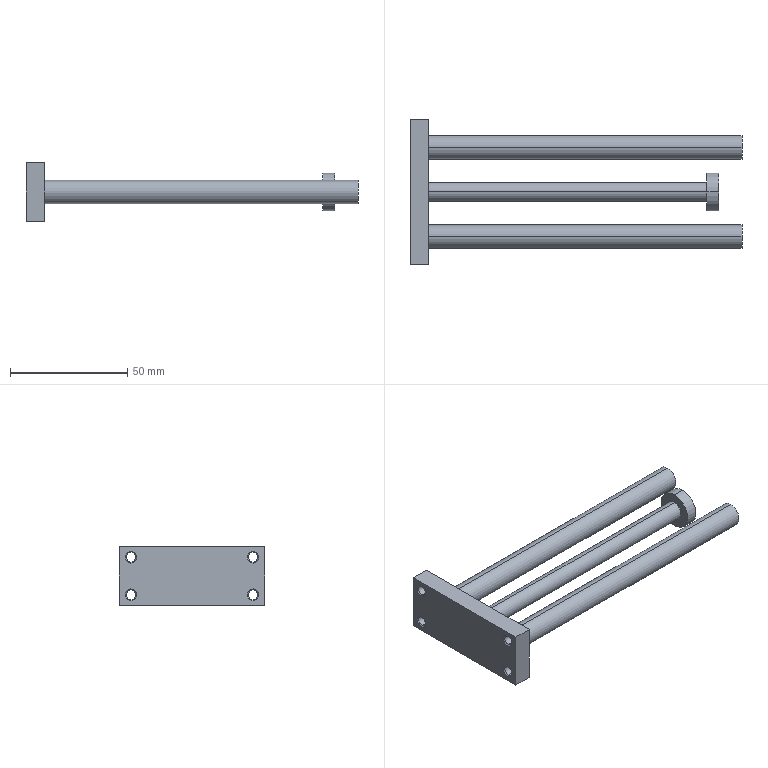Part | SolidWorks | features RefAxis 3, LPattern 2, Revolution 2, 3DProfileFeature 1, Extrusion 1, RevCut 1 | 1 solid | 42 faces | box 141.5 x 62 x 25 mm | volume 39892 mm3 | cylinder 16 | cone 16 | plane 10 | commonest cylinder face diameters 4.134 x8 10 x4 8 x2 16 x2
STEP:
#1=CARTESIAN_POINT('',(123.5,0.,8.));
#2=VERTEX_POINT('',#1);
#3=CARTESIAN_POINT('',(123.5,0.,-8.));
#4=VERTEX_POINT('',#3);
#5=CARTESIAN_POINT('',(123.5,0.,0.));
#6=DIRECTION('',(-1.,0.,0.));
#7=DIRECTION('',(0.,0.,1.));
#8=AXIS2_PLACEMENT_3D('',#5,#6,#7);
#9=CIRCLE('',#8,8.);
#10=EDGE_CURVE('',#2,#4,#9,.T.);
#11=ORIENTED_EDGE('',*,*,#10,.T.);
#12=CARTESIAN_POINT('',(118.5,0.,-8.));
#13=VERTEX_POINT('',#12);
#14=CARTESIAN_POINT('',(123.5,0.,-8.));
#15=DIRECTION('',(-1.,0.,0.));
#16=VECTOR('',#15,1000.);
#17=LINE('',#14,#16);
#18=EDGE_CURVE('',#4,#13,#17,.T.);
#19=ORIENTED_EDGE('',*,*,#18,.T.);
#20=CARTESIAN_POINT('',(118.5,0.,8.));
#21=VERTEX_POINT('',#20);
#22=CARTESIAN_POINT('',(118.5,0.,0.));
#23=DIRECTION('',(-1.,0.,0.));
#24=DIRECTION('',(0.,0.,1.));
#25=AXIS2_PLACEMENT_3D('',#22,#23,#24);
#26=CIRCLE('',#25,8.);
#27=EDGE_CURVE('',#21,#13,#26,.T.);
#28=ORIENTED_EDGE('',*,*,#27,.F.);
#29=CARTESIAN_POINT('',(123.5,0.,8.));
#30=DIRECTION('',(-1.,0.,0.));
#31=VECTOR('',#30,1000.);
#32=LINE('',#29,#31);
#33=EDGE_CURVE('',#2,#21,#32,.T.);
#34=ORIENTED_EDGE('',*,*,#33,.F.);
#35=EDGE_LOOP('',(#11,#19,#28,#34));
#36=FACE_OUTER_BOUND('',#35,.T.);
#37=CARTESIAN_POINT('',(123.5,0.,0.));
#38=DIRECTION('',(-1.,0.,0.));
#39=DIRECTION('',(0.,0.,1.));
#40=AXIS2_PLACEMENT_3D('',#37,#38,#39);
#41=CYLINDRICAL_SURFACE('',#40,8.);
#42=ADVANCED_FACE('',(#36),#41,.T.);
#43=CARTESIAN_POINT('',(118.5,0.,4.));
#44=VERTEX_POINT('',#43);
#45=CARTESIAN_POINT('',(118.5,0.,-4.));
#46=VERTEX_POINT('',#45);
#47=CARTESIAN_POINT('',(118.5,0.,0.));
#48=DIRECTION('',(-1.,0.,0.));
#49=DIRECTION('',(0.,0.,1.));
#50=AXIS2_PLACEMENT_3D('',#47,#48,#49);
#51=CIRCLE('',#50,4.);
#52=EDGE_CURVE('',#44,#46,#51,.T.);
#53=ORIENTED_EDGE('',*,*,#52,.T.);
#54=CARTESIAN_POINT('',(0.,0.,-4.));
#55=VERTEX_POINT('',#54);
#56=CARTESIAN_POINT('',(123.5,0.,-4.));
#57=DIRECTION('',(-1.,0.,0.));
#58=VECTOR('',#57,1000.);
#59=LINE('',#56,#58);
#60=EDGE_CURVE('',#46,#55,#59,.T.);
#61=ORIENTED_EDGE('',*,*,#60,.T.);
#62=CARTESIAN_POINT('',(0.,0.,4.));
#63=VERTEX_POINT('',#62);
#64=CARTESIAN_POINT('',(0.,0.,0.));
#65=DIRECTION('',(-1.,0.,0.));
#66=DIRECTION('',(0.,0.,1.));
#67=AXIS2_PLACEMENT_3D('',#64,#65,#66);
#68=CIRCLE('',#67,4.);
#69=EDGE_CURVE('',#63,#55,#68,.T.);
#70=ORIENTED_EDGE('',*,*,#69,.F.);
#71=CARTESIAN_POINT('',(123.5,0.,4.));
#72=DIRECTION('',(-1.,0.,0.));
#73=VECTOR('',#72,1000.);
#74=LINE('',#71,#73);
#75=EDGE_CURVE('',#44,#63,#74,.T.);
#76=ORIENTED_EDGE('',*,*,#75,.F.);
#77=EDGE_LOOP('',(#53,#61,#70,#76));
#78=FACE_OUTER_BOUND('',#77,.T.);
#79=CARTESIAN_POINT('',(123.5,0.,0.));
#80=DIRECTION('',(-1.,0.,0.));
#81=DIRECTION('',(0.,0.,1.));
#82=AXIS2_PLACEMENT_3D('',#79,#80,#81);
#83=CYLINDRICAL_SURFACE('',#82,4.);
#84=ADVANCED_FACE('',(#78),#83,.T.);
#85=CARTESIAN_POINT('',(-0.433,-26.,-10.067));
#86=VERTEX_POINT('',#85);
#87=CARTESIAN_POINT('',(-0.433,-26.,-5.933));
#88=VERTEX_POINT('',#87);
#89=CARTESIAN_POINT('',(-0.433,-26.,-8.));
#90=DIRECTION('',(-1.,0.,0.));
#91=DIRECTION('',(0.,0.,1.));
#92=AXIS2_PLACEMENT_3D('',#89,#90,#91);
#93=CIRCLE('',#92,2.067);
#94=EDGE_CURVE('',#86,#88,#93,.T.);
#95=ORIENTED_EDGE('',*,*,#94,.T.);
#96=CARTESIAN_POINT('',(0.,-26.,-5.5));
#97=VERTEX_POINT('',#96);
#98=CARTESIAN_POINT('',(0.,-26.,-5.5));
#99=DIRECTION('',(0.7071,0.,0.7071));
#100=VECTOR('',#99,1000.);
#101=LINE('',#98,#100);
#102=EDGE_CURVE('',#88,#97,#101,.T.);
#103=ORIENTED_EDGE('',*,*,#102,.T.);
#104=CARTESIAN_POINT('',(0.,-26.,-10.5));
#105=VERTEX_POINT('',#104);
#106=CARTESIAN_POINT('',(0.,-26.,-8.));
#107=DIRECTION('',(-1.,0.,0.));
#108=DIRECTION('',(0.,0.,1.));
#109=AXIS2_PLACEMENT_3D('',#106,#107,#108);
#110=CIRCLE('',#109,2.5);
#111=EDGE_CURVE('',#105,#97,#110,.T.);
#112=ORIENTED_EDGE('',*,*,#111,.F.);
#113=CARTESIAN_POINT('',(0.,-26.,-10.5));
#114=DIRECTION('',(0.7071,0.,-0.7071));
#115=VECTOR('',#114,1000.);
#116=LINE('',#113,#115);
#117=EDGE_CURVE('',#86,#105,#116,.T.);
#118=ORIENTED_EDGE('',*,*,#117,.F.);
#119=EDGE_LOOP('',(#95,#103,#112,#118));
#120=FACE_OUTER_BOUND('',#119,.T.);
#121=CARTESIAN_POINT('',(0.,-26.,-8.));
#122=DIRECTION('',(1.,0.,0.));
#123=DIRECTION('',(0.,0.,-1.));
#124=AXIS2_PLACEMENT_3D('',#121,#122,#123);
#125=CONICAL_SURFACE('',#124,2.5,0.7854);
#126=ADVANCED_FACE('',(#120),#125,.F.);
#127=ORIENTED_EDGE('',*,*,#94,.F.);
#128=CARTESIAN_POINT('',(-7.567,-26.,-10.067));
#129=VERTEX_POINT('',#128);
#130=CARTESIAN_POINT('',(0.,-26.,-10.067));
#131=DIRECTION('',(-1.,0.,0.));
#132=VECTOR('',#131,1000.);
#133=LINE('',#130,#132);
#134=EDGE_CURVE('',#86,#129,#133,.T.);
#135=ORIENTED_EDGE('',*,*,#134,.T.);
#136=CARTESIAN_POINT('',(-7.567,-26.,-5.933));
#137=VERTEX_POINT('',#136);
#138=CARTESIAN_POINT('',(-7.567,-26.,-8.));
#139=DIRECTION('',(-1.,0.,0.));
#140=DIRECTION('',(0.,0.,1.));
#141=AXIS2_PLACEMENT_3D('',#138,#139,#140);
#142=CIRCLE('',#141,2.067);
#143=EDGE_CURVE('',#129,#137,#142,.T.);
#144=ORIENTED_EDGE('',*,*,#143,.T.);
#145=CARTESIAN_POINT('',(0.,-26.,-5.933));
#146=DIRECTION('',(-1.,0.,0.));
#147=VECTOR('',#146,1000.);
#148=LINE('',#145,#147);
#149=EDGE_CURVE('',#88,#137,#148,.T.);
#150=ORIENTED_EDGE('',*,*,#149,.F.);
#151=EDGE_LOOP('',(#127,#135,#144,#150));
#152=FACE_OUTER_BOUND('',#151,.T.);
#153=CARTESIAN_POINT('',(0.,-26.,-8.));
#154=DIRECTION('',(-1.,0.,0.));
#155=DIRECTION('',(0.,0.,1.));
#156=AXIS2_PLACEMENT_3D('',#153,#154,#155);
#157=CYLINDRICAL_SURFACE('',#156,2.067);
#158=ADVANCED_FACE('',(#152),#157,.F.);
#159=ORIENTED_EDGE('',*,*,#143,.F.);
#160=CARTESIAN_POINT('',(-8.,-26.,-10.5));
#161=VERTEX_POINT('',#160);
#162=CARTESIAN_POINT('',(-7.567,-26.,-10.067));
#163=DIRECTION('',(-0.7071,0.,-0.7071));
#164=VECTOR('',#163,1000.);
#165=LINE('',#162,#164);
#166=EDGE_CURVE('',#129,#161,#165,.T.);
#167=ORIENTED_EDGE('',*,*,#166,.T.);
#168=CARTESIAN_POINT('',(-8.,-26.,-5.5));
#169=VERTEX_POINT('',#168);
#170=CARTESIAN_POINT('',(-8.,-26.,-8.));
#171=DIRECTION('',(-1.,0.,0.));
#172=DIRECTION('',(0.,0.,1.));
#173=AXIS2_PLACEMENT_3D('',#170,#171,#172);
#174=CIRCLE('',#173,2.5);
#175=EDGE_CURVE('',#161,#169,#174,.T.);
#176=ORIENTED_EDGE('',*,*,#175,.T.);
#177=CARTESIAN_POINT('',(-7.567,-26.,-5.933));
#178=DIRECTION('',(-0.7071,0.,0.7071));
#179=VECTOR('',#178,1000.);
#180=LINE('',#177,#179);
#181=EDGE_CURVE('',#137,#169,#180,.T.);
#182=ORIENTED_EDGE('',*,*,#181,.F.);
#183=EDGE_LOOP('',(#159,#167,#176,#182));
#184=FACE_OUTER_BOUND('',#183,.T.);
#185=CARTESIAN_POINT('',(-7.567,-26.,-8.));
#186=DIRECTION('',(-1.,0.,0.));
#187=DIRECTION('',(0.,0.,1.));
#188=AXIS2_PLACEMENT_3D('',#185,#186,#187);
#189=CONICAL_SURFACE('',#188,2.067,0.7854);
#190=ADVANCED_FACE('',(#184),#189,.F.);
#191=CARTESIAN_POINT('',(-0.433,26.,-10.067));
#192=VERTEX_POINT('',#191);
#193=CARTESIAN_POINT('',(-0.433,26.,-5.933));
#194=VERTEX_POINT('',#193);
#195=CARTESIAN_POINT('',(-0.433,26.,-8.));
#196=DIRECTION('',(-1.,0.,0.));
#197=DIRECTION('',(0.,0.,1.));
#198=AXIS2_PLACEMENT_3D('',#195,#196,#197);
#199=CIRCLE('',#198,2.067);
#200=EDGE_CURVE('',#192,#194,#199,.T.);
#201=ORIENTED_EDGE('',*,*,#200,.T.);
#202=CARTESIAN_POINT('',(0.,26.,-5.5));
#203=VERTEX_POINT('',#202);
#204=CARTESIAN_POINT('',(0.,26.,-5.5));
#205=DIRECTION('',(0.7071,0.,0.7071));
#206=VECTOR('',#205,1000.);
#207=LINE('',#204,#206);
#208=EDGE_CURVE('',#194,#203,#207,.T.);
#209=ORIENTED_EDGE('',*,*,#208,.T.);
#210=CARTESIAN_POINT('',(0.,26.,-10.5));
#211=VERTEX_POINT('',#210);
#212=CARTESIAN_POINT('',(0.,26.,-8.));
#213=DIRECTION('',(-1.,0.,0.));
#214=DIRECTION('',(0.,0.,1.));
#215=AXIS2_PLACEMENT_3D('',#212,#213,#214);
#216=CIRCLE('',#215,2.5);
#217=EDGE_CURVE('',#211,#203,#216,.T.);
#218=ORIENTED_EDGE('',*,*,#217,.F.);
#219=CARTESIAN_POINT('',(0.,26.,-10.5));
#220=DIRECTION('',(0.7071,0.,-0.7071));
#221=VECTOR('',#220,1000.);
#222=LINE('',#219,#221);
#223=EDGE_CURVE('',#192,#211,#222,.T.);
#224=ORIENTED_EDGE('',*,*,#223,.F.);
#225=EDGE_LOOP('',(#201,#209,#218,#224));
#226=FACE_OUTER_BOUND('',#225,.T.);
#227=CARTESIAN_POINT('',(0.,26.,-8.));
#228=DIRECTION('',(1.,0.,0.));
#229=DIRECTION('',(0.,0.,-1.));
#230=AXIS2_PLACEMENT_3D('',#227,#228,#229);
#231=CONICAL_SURFACE('',#230,2.5,0.7854);
#232=ADVANCED_FACE('',(#226),#231,.F.);
#233=ORIENTED_EDGE('',*,*,#200,.F.);
#234=CARTESIAN_POINT('',(-7.567,26.,-10.067));
#235=VERTEX_POINT('',#234);
#236=CARTESIAN_POINT('',(0.,26.,-10.067));
#237=DIRECTION('',(-1.,0.,0.));
#238=VECTOR('',#237,1000.);
#239=LINE('',#236,#238);
#240=EDGE_CURVE('',#192,#235,#239,.T.);
#241=ORIENTED_EDGE('',*,*,#240,.T.);
#242=CARTESIAN_POINT('',(-7.567,26.,-5.933));
#243=VERTEX_POINT('',#242);
#244=CARTESIAN_POINT('',(-7.567,26.,-8.));
#245=DIRECTION('',(-1.,0.,0.));
#246=DIRECTION('',(0.,0.,1.));
#247=AXIS2_PLACEMENT_3D('',#244,#245,#246);
#248=CIRCLE('',#247,2.067);
#249=EDGE_CURVE('',#235,#243,#248,.T.);
#250=ORIENTED_EDGE('',*,*,#249,.T.);
#251=CARTESIAN_POINT('',(0.,26.,-5.933));
#252=DIRECTION('',(-1.,0.,0.));
#253=VECTOR('',#252,1000.);
#254=LINE('',#251,#253);
#255=EDGE_CURVE('',#194,#243,#254,.T.);
#256=ORIENTED_EDGE('',*,*,#255,.F.);
#257=EDGE_LOOP('',(#233,#241,#250,#256));
#258=FACE_OUTER_BOUND('',#257,.T.);
#259=CARTESIAN_POINT('',(0.,26.,-8.));
#260=DIRECTION('',(-1.,0.,0.));
#261=DIRECTION('',(0.,0.,1.));
#262=AXIS2_PLACEMENT_3D('',#259,#260,#261);
#263=CYLINDRICAL_SURFACE('',#262,2.067);
#264=ADVANCED_FACE('',(#258),#263,.F.);
#265=ORIENTED_EDGE('',*,*,#249,.F.);
#266=CARTESIAN_POINT('',(-8.,26.,-10.5));
#267=VERTEX_POINT('',#266);
#268=CARTESIAN_POINT('',(-7.567,26.,-10.067));
#269=DIRECTION('',(-0.7071,0.,-0.7071));
#270=VECTOR('',#269,1000.);
#271=LINE('',#268,#270);
#272=EDGE_CURVE('',#235,#267,#271,.T.);
#273=ORIENTED_EDGE('',*,*,#272,.T.);
#274=CARTESIAN_POINT('',(-8.,26.,-5.5));
#275=VERTEX_POINT('',#274);
#276=CARTESIAN_POINT('',(-8.,26.,-8.));
#277=DIRECTION('',(-1.,0.,0.));
#278=DIRECTION('',(0.,0.,1.));
#279=AXIS2_PLACEMENT_3D('',#276,#277,#278);
#280=CIRCLE('',#279,2.5);
#281=EDGE_CURVE('',#267,#275,#280,.T.);
#282=ORIENTED_EDGE('',*,*,#281,.T.);
#283=CARTESIAN_POINT('',(-7.567,26.,-5.933));
#284=DIRECTION('',(-0.7071,0.,0.7071));
#285=VECTOR('',#284,1000.);
#286=LINE('',#283,#285);
#287=EDGE_CURVE('',#243,#275,#286,.T.);
#288=ORIENTED_EDGE('',*,*,#287,.F.);
#289=EDGE_LOOP('',(#265,#273,#282,#288));
#290=FACE_OUTER_BOUND('',#289,.T.);
#291=CARTESIAN_POINT('',(-7.567,26.,-8.));
#292=DIRECTION('',(-1.,0.,0.));
#293=DIRECTION('',(0.,0.,1.));
#294=AXIS2_PLACEMENT_3D('',#291,#292,#293);
#295=CONICAL_SURFACE('',#294,2.067,0.7854);
#296=ADVANCED_FACE('',(#290),#295,.F.);
#297=CARTESIAN_POINT('',(-0.433,-26.,5.933));
#298=VERTEX_POINT('',#297);
#299=CARTESIAN_POINT('',(-0.433,-26.,10.067));
#300=VERTEX_POINT('',#299);
#301=CARTESIAN_POINT('',(-0.433,-26.,8.));
#302=DIRECTION('',(-1.,0.,0.));
#303=DIRECTION('',(0.,0.,1.));
#304=AXIS2_PLACEMENT_3D('',#301,#302,#303);
#305=CIRCLE('',#304,2.067);
#306=EDGE_CURVE('',#298,#300,#305,.T.);
#307=ORIENTED_EDGE('',*,*,#306,.T.);
#308=CARTESIAN_POINT('',(0.,-26.,10.5));
#309=VERTEX_POINT('',#308);
#310=CARTESIAN_POINT('',(0.,-26.,10.5));
#311=DIRECTION('',(0.7071,0.,0.7071));
#312=VECTOR('',#311,1000.);
#313=LINE('',#310,#312);
#314=EDGE_CURVE('',#300,#309,#313,.T.);
#315=ORIENTED_EDGE('',*,*,#314,.T.);
#316=CARTESIAN_POINT('',(0.,-26.,5.5));
#317=VERTEX_POINT('',#316);
#318=CARTESIAN_POINT('',(0.,-26.,8.));
#319=DIRECTION('',(-1.,0.,0.));
#320=DIRECTION('',(0.,0.,1.));
#321=AXIS2_PLACEMENT_3D('',#318,#319,#320);
#322=CIRCLE('',#321,2.5);
#323=EDGE_CURVE('',#317,#309,#322,.T.);
#324=ORIENTED_EDGE('',*,*,#323,.F.);
#325=CARTESIAN_POINT('',(0.,-26.,5.5));
#326=DIRECTION('',(0.7071,0.,-0.7071));
#327=VECTOR('',#326,1000.);
#328=LINE('',#325,#327);
#329=EDGE_CURVE('',#298,#317,#328,.T.);
#330=ORIENTED_EDGE('',*,*,#329,.F.);
#331=EDGE_LOOP('',(#307,#315,#324,#330));
#332=FACE_OUTER_BOUND('',#331,.T.);
#333=CARTESIAN_POINT('',(0.,-26.,8.));
#334=DIRECTION('',(1.,0.,0.));
#335=DIRECTION('',(0.,0.,-1.));
#336=AXIS2_PLACEMENT_3D('',#333,#334,#335);
#337=CONICAL_SURFACE('',#336,2.5,0.7854);
#338=ADVANCED_FACE('',(#332),#337,.F.);
#339=ORIENTED_EDGE('',*,*,#306,.F.);
#340=CARTESIAN_POINT('',(-7.567,-26.,5.933));
#341=VERTEX_POINT('',#340);
#342=CARTESIAN_POINT('',(0.,-26.,5.933));
#343=DIRECTION('',(-1.,0.,0.));
#344=VECTOR('',#343,1000.);
#345=LINE('',#342,#344);
#346=EDGE_CURVE('',#298,#341,#345,.T.);
#347=ORIENTED_EDGE('',*,*,#346,.T.);
#348=CARTESIAN_POINT('',(-7.567,-26.,10.067));
#349=VERTEX_POINT('',#348);
#350=CARTESIAN_POINT('',(-7.567,-26.,8.));
#351=DIRECTION('',(-1.,0.,0.));
#352=DIRECTION('',(0.,0.,1.));
#353=AXIS2_PLACEMENT_3D('',#350,#351,#352);
#354=CIRCLE('',#353,2.067);
#355=EDGE_CURVE('',#341,#349,#354,.T.);
#356=ORIENTED_EDGE('',*,*,#355,.T.);
#357=CARTESIAN_POINT('',(0.,-26.,10.067));
#358=DIRECTION('',(-1.,0.,0.));
#359=VECTOR('',#358,1000.);
#360=LINE('',#357,#359);
#361=EDGE_CURVE('',#300,#349,#360,.T.);
#362=ORIENTED_EDGE('',*,*,#361,.F.);
#363=EDGE_LOOP('',(#339,#347,#356,#362));
#364=FACE_OUTER_BOUND('',#363,.T.);
#365=CARTESIAN_POINT('',(0.,-26.,8.));
#366=DIRECTION('',(-1.,0.,0.));
#367=DIRECTION('',(0.,0.,1.));
#368=AXIS2_PLACEMENT_3D('',#365,#366,#367);
#369=CYLINDRICAL_SURFACE('',#368,2.067);
#370=ADVANCED_FACE('',(#364),#369,.F.);
#371=ORIENTED_EDGE('',*,*,#355,.F.);
#372=CARTESIAN_POINT('',(-8.,-26.,5.5));
#373=VERTEX_POINT('',#372);
#374=CARTESIAN_POINT('',(-7.567,-26.,5.933));
#375=DIRECTION('',(-0.7071,0.,-0.7071));
#376=VECTOR('',#375,1000.);
#377=LINE('',#374,#376);
#378=EDGE_CURVE('',#341,#373,#377,.T.);
#379=ORIENTED_EDGE('',*,*,#378,.T.);
#380=CARTESIAN_POINT('',(-8.,-26.,10.5));
#381=VERTEX_POINT('',#380);
#382=CARTESIAN_POINT('',(-8.,-26.,8.));
#383=DIRECTION('',(-1.,0.,0.));
#384=DIRECTION('',(0.,0.,1.));
#385=AXIS2_PLACEMENT_3D('',#382,#383,#384);
#386=CIRCLE('',#385,2.5);
#387=EDGE_CURVE('',#373,#381,#386,.T.);
#388=ORIENTED_EDGE('',*,*,#387,.T.);
#389=CARTESIAN_POINT('',(-7.567,-26.,10.067));
#390=DIRECTION('',(-0.7071,0.,0.7071));
#391=VECTOR('',#390,1000.);
#392=LINE('',#389,#391);
#393=EDGE_CURVE('',#349,#381,#392,.T.);
#394=ORIENTED_EDGE('',*,*,#393,.F.);
#395=EDGE_LOOP('',(#371,#379,#388,#394));
#396=FACE_OUTER_BOUND('',#395,.T.);
#397=CARTESIAN_POINT('',(-7.567,-26.,8.));
#398=DIRECTION('',(-1.,0.,0.));
#399=DIRECTION('',(0.,0.,1.));
#400=AXIS2_PLACEMENT_3D('',#397,#398,#399);
#401=CONICAL_SURFACE('',#400,2.067,0.7854);
#402=ADVANCED_FACE('',(#396),#401,.F.);
#403=CARTESIAN_POINT('',(-0.433,26.,5.933));
#404=VERTEX_POINT('',#403);
#405=CARTESIAN_POINT('',(-0.433,26.,10.067));
#406=VERTEX_POINT('',#405);
#407=CARTESIAN_POINT('',(-0.433,26.,8.));
#408=DIRECTION('',(-1.,0.,0.));
#409=DIRECTION('',(0.,0.,1.));
#410=AXIS2_PLACEMENT_3D('',#407,#408,#409);
#411=CIRCLE('',#410,2.067);
#412=EDGE_CURVE('',#404,#406,#411,.T.);
#413=ORIENTED_EDGE('',*,*,#412,.T.);
#414=CARTESIAN_POINT('',(0.,26.,10.5));
#415=VERTEX_POINT('',#414);
#416=CARTESIAN_POINT('',(0.,26.,10.5));
#417=DIRECTION('',(0.7071,0.,0.7071));
#418=VECTOR('',#417,1000.);
#419=LINE('',#416,#418);
#420=EDGE_CURVE('',#406,#415,#419,.T.);
#421=ORIENTED_EDGE('',*,*,#420,.T.);
#422=CARTESIAN_POINT('',(0.,26.,5.5));
#423=VERTEX_POINT('',#422);
#424=CARTESIAN_POINT('',(0.,26.,8.));
#425=DIRECTION('',(-1.,0.,0.));
#426=DIRECTION('',(0.,0.,1.));
#427=AXIS2_PLACEMENT_3D('',#424,#425,#426);
#428=CIRCLE('',#427,2.5);
#429=EDGE_CURVE('',#423,#415,#428,.T.);
#430=ORIENTED_EDGE('',*,*,#429,.F.);
#431=CARTESIAN_POINT('',(0.,26.,5.5));
#432=DIRECTION('',(0.7071,0.,-0.7071));
#433=VECTOR('',#432,1000.);
#434=LINE('',#431,#433);
#435=EDGE_CURVE('',#404,#423,#434,.T.);
#436=ORIENTED_EDGE('',*,*,#435,.F.);
#437=EDGE_LOOP('',(#413,#421,#430,#436));
#438=FACE_OUTER_BOUND('',#437,.T.);
#439=CARTESIAN_POINT('',(0.,26.,8.));
#440=DIRECTION('',(1.,0.,0.));
#441=DIRECTION('',(0.,0.,-1.));
#442=AXIS2_PLACEMENT_3D('',#439,#440,#441);
#443=CONICAL_SURFACE('',#442,2.5,0.7854);
#444=ADVANCED_FACE('',(#438),#443,.F.);
#445=ORIENTED_EDGE('',*,*,#412,.F.);
#446=CARTESIAN_POINT('',(-7.567,26.,5.933));
#447=VERTEX_POINT('',#446);
#448=CARTESIAN_POINT('',(0.,26.,5.933));
#449=DIRECTION('',(-1.,0.,0.));
#450=VECTOR('',#449,1000.);
#451=LINE('',#448,#450);
#452=EDGE_CURVE('',#404,#447,#451,.T.);
#453=ORIENTED_EDGE('',*,*,#452,.T.);
#454=CARTESIAN_POINT('',(-7.567,26.,10.067));
#455=VERTEX_POINT('',#454);
#456=CARTESIAN_POINT('',(-7.567,26.,8.));
#457=DIRECTION('',(-1.,0.,0.));
#458=DIRECTION('',(0.,0.,1.));
#459=AXIS2_PLACEMENT_3D('',#456,#457,#458);
#460=CIRCLE('',#459,2.067);
#461=EDGE_CURVE('',#447,#455,#460,.T.);
#462=ORIENTED_EDGE('',*,*,#461,.T.);
#463=CARTESIAN_POINT('',(0.,26.,10.067));
#464=DIRECTION('',(-1.,0.,0.));
#465=VECTOR('',#464,1000.);
#466=LINE('',#463,#465);
#467=EDGE_CURVE('',#406,#455,#466,.T.);
#468=ORIENTED_EDGE('',*,*,#467,.F.);
#469=EDGE_LOOP('',(#445,#453,#462,#468));
#470=FACE_OUTER_BOUND('',#469,.T.);
#471=CARTESIAN_POINT('',(0.,26.,8.));
#472=DIRECTION('',(-1.,0.,0.));
#473=DIRECTION('',(0.,0.,1.));
#474=AXIS2_PLACEMENT_3D('',#471,#472,#473);
#475=CYLINDRICAL_SURFACE('',#474,2.067);
#476=ADVANCED_FACE('',(#470),#475,.F.);
#477=ORIENTED_EDGE('',*,*,#461,.F.);
#478=CARTESIAN_POINT('',(-8.,26.,5.5));
#479=VERTEX_POINT('',#478);
#480=CARTESIAN_POINT('',(-7.567,26.,5.933));
#481=DIRECTION('',(-0.7071,0.,-0.7071));
#482=VECTOR('',#481,1000.);
#483=LINE('',#480,#482);
#484=EDGE_CURVE('',#447,#479,#483,.T.);
#485=ORIENTED_EDGE('',*,*,#484,.T.);
#486=CARTESIAN_POINT('',(-8.,26.,10.5));
#487=VERTEX_POINT('',#486);
#488=CARTESIAN_POINT('',(-8.,26.,8.));
#489=DIRECTION('',(-1.,0.,0.));
#490=DIRECTION('',(0.,0.,1.));
#491=AXIS2_PLACEMENT_3D('',#488,#489,#490);
#492=CIRCLE('',#491,2.5);
#493=EDGE_CURVE('',#479,#487,#492,.T.);
#494=ORIENTED_EDGE('',*,*,#493,.T.);
#495=CARTESIAN_POINT('',(-7.567,26.,10.067));
#496=DIRECTION('',(-0.7071,0.,0.7071));
#497=VECTOR('',#496,1000.);
#498=LINE('',#495,#497);
#499=EDGE_CURVE('',#455,#487,#498,.T.);
#500=ORIENTED_EDGE('',*,*,#499,.F.);
#501=EDGE_LOOP('',(#477,#485,#494,#500));
#502=FACE_OUTER_BOUND('',#501,.T.);
#503=CARTESIAN_POINT('',(-7.567,26.,8.));
#504=DIRECTION('',(-1.,0.,0.));
#505=DIRECTION('',(0.,0.,1.));
#506=AXIS2_PLACEMENT_3D('',#503,#504,#505);
#507=CONICAL_SURFACE('',#506,2.067,0.7854);
#508=ADVANCED_FACE('',(#502),#507,.F.);
#509=CARTESIAN_POINT('',(133.5,-19.,5.));
#510=VERTEX_POINT('',#509);
#511=CARTESIAN_POINT('',(133.5,-19.,-5.));
#512=VERTEX_POINT('',#511);
#513=CARTESIAN_POINT('',(133.5,-19.,0.));
#514=DIRECTION('',(-1.,0.,0.));
#515=DIRECTION('',(0.,0.,1.));
#516=AXIS2_PLACEMENT_3D('',#513,#514,#515);
#517=CIRCLE('',#516,5.);
#518=EDGE_CURVE('',#510,#512,#517,.T.);
#519=ORIENTED_EDGE('',*,*,#518,.T.);
#520=CARTESIAN_POINT('',(0.,-19.,-5.));
#521=VERTEX_POINT('',#520);
#522=CARTESIAN_POINT('',(133.5,-19.,-5.));
#523=DIRECTION('',(-1.,0.,0.));
#524=VECTOR('',#523,1000.);
#525=LINE('',#522,#524);
#526=EDGE_CURVE('',#512,#521,#525,.T.);
#527=ORIENTED_EDGE('',*,*,#526,.T.);
#528=CARTESIAN_POINT('',(0.,-19.,5.));
#529=VERTEX_POINT('',#528);
#530=CARTESIAN_POINT('',(0.,-19.,0.));
#531=DIRECTION('',(-1.,0.,0.));
#532=DIRECTION('',(0.,0.,1.));
#533=AXIS2_PLACEMENT_3D('',#530,#531,#532);
#534=CIRCLE('',#533,5.);
#535=EDGE_CURVE('',#529,#521,#534,.T.);
#536=ORIENTED_EDGE('',*,*,#535,.F.);
#537=CARTESIAN_POINT('',(133.5,-19.,5.));
#538=DIRECTION('',(-1.,0.,0.));
#539=VECTOR('',#538,1000.);
#540=LINE('',#537,#539);
#541=EDGE_CURVE('',#510,#529,#540,.T.);
#542=ORIENTED_EDGE('',*,*,#541,.F.);
#543=EDGE_LOOP('',(#519,#527,#536,#542));
#544=FACE_OUTER_BOUND('',#543,.T.);
#545=CARTESIAN_POINT('',(133.5,-19.,0.));
#546=DIRECTION('',(-1.,0.,0.));
#547=DIRECTION('',(0.,0.,1.));
#548=AXIS2_PLACEMENT_3D('',#545,#546,#547);
#549=CYLINDRICAL_SURFACE('',#548,5.);
#550=ADVANCED_FACE('',(#544),#549,.T.);
#551=CARTESIAN_POINT('',(133.5,19.,5.));
#552=VERTEX_POINT('',#551);
#553=CARTESIAN_POINT('',(133.5,19.,-5.));
#554=VERTEX_POINT('',#553);
#555=CARTESIAN_POINT('',(133.5,19.,0.));
#556=DIRECTION('',(-1.,0.,0.));
#557=DIRECTION('',(0.,0.,1.));
#558=AXIS2_PLACEMENT_3D('',#555,#556,#557);
#559=CIRCLE('',#558,5.);
#560=EDGE_CURVE('',#552,#554,#559,.T.);
#561=ORIENTED_EDGE('',*,*,#560,.T.);
#562=CARTESIAN_POINT('',(0.,19.,-5.));
#563=VERTEX_POINT('',#562);
#564=CARTESIAN_POINT('',(133.5,19.,-5.));
#565=DIRECTION('',(-1.,0.,0.));
#566=VECTOR('',#565,1000.);
#567=LINE('',#564,#566);
#568=EDGE_CURVE('',#554,#563,#567,.T.);
#569=ORIENTED_EDGE('',*,*,#568,.T.);
#570=CARTESIAN_POINT('',(0.,19.,5.));
#571=VERTEX_POINT('',#570);
#572=CARTESIAN_POINT('',(0.,19.,0.));
#573=DIRECTION('',(-1.,0.,0.));
#574=DIRECTION('',(0.,0.,1.));
#575=AXIS2_PLACEMENT_3D('',#572,#573,#574);
#576=CIRCLE('',#575,5.);
#577=EDGE_CURVE('',#571,#563,#576,.T.);
#578=ORIENTED_EDGE('',*,*,#577,.F.);
#579=CARTESIAN_POINT('',(133.5,19.,5.));
#580=DIRECTION('',(-1.,0.,0.));
#581=VECTOR('',#580,1000.);
#582=LINE('',#579,#581);
#583=EDGE_CURVE('',#552,#571,#582,.T.);
#584=ORIENTED_EDGE('',*,*,#583,.F.);
#585=EDGE_LOOP('',(#561,#569,#578,#584));
#586=FACE_OUTER_BOUND('',#585,.T.);
#587=CARTESIAN_POINT('',(133.5,19.,0.));
#588=DIRECTION('',(-1.,0.,0.));
#589=DIRECTION('',(0.,0.,1.));
#590=AXIS2_PLACEMENT_3D('',#587,#588,#589);
#591=CYLINDRICAL_SURFACE('',#590,5.);
#592=ADVANCED_FACE('',(#586),#591,.T.);
#593=ORIENTED_EDGE('',*,*,#111,.T.);
#594=CARTESIAN_POINT('',(0.,-26.,-8.));
#595=DIRECTION('',(-1.,0.,0.));
#596=DIRECTION('',(0.,0.,1.));
#597=AXIS2_PLACEMENT_3D('',#594,#595,#596);
#598=CIRCLE('',#597,2.5);
#599=EDGE_CURVE('',#97,#105,#598,.T.);
#600=ORIENTED_EDGE('',*,*,#599,.T.);
#601=EDGE_LOOP('',(#593,#600));
#602=FACE_BOUND('',#601,.T.);
#603=ORIENTED_EDGE('',*,*,#323,.T.);
#604=CARTESIAN_POINT('',(0.,-26.,8.));
#605=DIRECTION('',(-1.,0.,0.));
#606=DIRECTION('',(0.,0.,1.));
#607=AXIS2_PLACEMENT_3D('',#604,#605,#606);
#608=CIRCLE('',#607,2.5);
#609=EDGE_CURVE('',#309,#317,#608,.T.);
#610=ORIENTED_EDGE('',*,*,#609,.T.);
#611=EDGE_LOOP('',(#603,#610));
#612=FACE_BOUND('',#611,.T.);
#613=ORIENTED_EDGE('',*,*,#535,.T.);
#614=CARTESIAN_POINT('',(0.,-19.,0.));
#615=DIRECTION('',(-1.,0.,0.));
#616=DIRECTION('',(0.,0.,1.));
#617=AXIS2_PLACEMENT_3D('',#614,#615,#616);
#618=CIRCLE('',#617,5.);
#619=EDGE_CURVE('',#521,#529,#618,.T.);
#620=ORIENTED_EDGE('',*,*,#619,.T.);
#621=EDGE_LOOP('',(#613,#620));
#622=FACE_BOUND('',#621,.T.);
#623=CARTESIAN_POINT('',(0.,31.,12.5));
#624=VERTEX_POINT('',#623);
#625=CARTESIAN_POINT('',(0.,-31.,12.5));
#626=VERTEX_POINT('',#625);
#627=CARTESIAN_POINT('',(0.,31.,12.5));
#628=DIRECTION('',(0.,-1.,0.));
#629=VECTOR('',#628,1000.);
#630=LINE('',#627,#629);
#631=EDGE_CURVE('',#624,#626,#630,.T.);
#632=ORIENTED_EDGE('',*,*,#631,.T.);
#633=CARTESIAN_POINT('',(0.,-31.,-12.5));
#634=VERTEX_POINT('',#633);
#635=CARTESIAN_POINT('',(0.,-31.,12.5));
#636=DIRECTION('',(0.,0.,-1.));
#637=VECTOR('',#636,1000.);
#638=LINE('',#635,#637);
#639=EDGE_CURVE('',#626,#634,#638,.T.);
#640=ORIENTED_EDGE('',*,*,#639,.T.);
#641=CARTESIAN_POINT('',(0.,31.,-12.5));
#642=VERTEX_POINT('',#641);
#643=CARTESIAN_POINT('',(0.,-31.,-12.5));
#644=DIRECTION('',(0.,1.,0.));
#645=VECTOR('',#644,1000.);
#646=LINE('',#643,#645);
#647=EDGE_CURVE('',#634,#642,#646,.T.);
#648=ORIENTED_EDGE('',*,*,#647,.T.);
#649=CARTESIAN_POINT('',(0.,31.,-12.5));
#650=DIRECTION('',(0.,0.,1.));
#651=VECTOR('',#650,1000.);
#652=LINE('',#649,#651);
#653=EDGE_CURVE('',#642,#624,#652,.T.);
#654=ORIENTED_EDGE('',*,*,#653,.T.);
#655=EDGE_LOOP('',(#632,#640,#648,#654));
#656=FACE_OUTER_BOUND('',#655,.T.);
#657=ORIENTED_EDGE('',*,*,#577,.T.);
#658=CARTESIAN_POINT('',(0.,19.,0.));
#659=DIRECTION('',(-1.,0.,0.));
#660=DIRECTION('',(0.,0.,1.));
#661=AXIS2_PLACEMENT_3D('',#658,#659,#660);
#662=CIRCLE('',#661,5.);
#663=EDGE_CURVE('',#563,#571,#662,.T.);
#664=ORIENTED_EDGE('',*,*,#663,.T.);
#665=EDGE_LOOP('',(#657,#664));
#666=FACE_BOUND('',#665,.T.);
#667=ORIENTED_EDGE('',*,*,#429,.T.);
#668=CARTESIAN_POINT('',(0.,26.,8.));
#669=DIRECTION('',(-1.,0.,0.));
#670=DIRECTION('',(0.,0.,1.));
#671=AXIS2_PLACEMENT_3D('',#668,#669,#670);
#672=CIRCLE('',#671,2.5);
#673=EDGE_CURVE('',#415,#423,#672,.T.);
#674=ORIENTED_EDGE('',*,*,#673,.T.);
#675=EDGE_LOOP('',(#667,#674));
#676=FACE_BOUND('',#675,.T.);
#677=ORIENTED_EDGE('',*,*,#217,.T.);
#678=CARTESIAN_POINT('',(0.,26.,-8.));
#679=DIRECTION('',(-1.,0.,0.));
#680=DIRECTION('',(0.,0.,1.));
#681=AXIS2_PLACEMENT_3D('',#678,#679,#680);
#682=CIRCLE('',#681,2.5);
#683=EDGE_CURVE('',#203,#211,#682,.T.);
#684=ORIENTED_EDGE('',*,*,#683,.T.);
#685=EDGE_LOOP('',(#677,#684));
#686=FACE_BOUND('',#685,.T.);
#687=ORIENTED_EDGE('',*,*,#69,.T.);
#688=CARTESIAN_POINT('',(0.,0.,0.));
#689=DIRECTION('',(-1.,0.,0.));
#690=DIRECTION('',(0.,0.,1.));
#691=AXIS2_PLACEMENT_3D('',#688,#689,#690);
#692=CIRCLE('',#691,4.);
#693=EDGE_CURVE('',#55,#63,#692,.T.);
#694=ORIENTED_EDGE('',*,*,#693,.T.);
#695=EDGE_LOOP('',(#687,#694));
#696=FACE_BOUND('',#695,.T.);
#697=CARTESIAN_POINT('',(0.,0.,0.));
#698=DIRECTION('',(1.,0.,0.));
#699=DIRECTION('',(0.,0.,-1.));
#700=AXIS2_PLACEMENT_3D('',#697,#698,#699);
#701=PLANE('',#700);
#702=ADVANCED_FACE('',(#602,#612,#622,#656,#666,#676,#686,#696),#701,.T.);
#703=CARTESIAN_POINT('',(-8.,26.,-8.));
#704=DIRECTION('',(-1.,0.,0.));
#705=DIRECTION('',(0.,0.,1.));
#706=AXIS2_PLACEMENT_3D('',#703,#704,#705);
#707=CIRCLE('',#706,2.5);
#708=EDGE_CURVE('',#275,#267,#707,.T.);
#709=ORIENTED_EDGE('',*,*,#708,.F.);
#710=ORIENTED_EDGE('',*,*,#281,.F.);
#711=EDGE_LOOP('',(#709,#710));
#712=FACE_BOUND('',#711,.T.);
#713=CARTESIAN_POINT('',(-8.,26.,8.));
#714=DIRECTION('',(-1.,0.,0.));
#715=DIRECTION('',(0.,0.,1.));
#716=AXIS2_PLACEMENT_3D('',#713,#714,#715);
#717=CIRCLE('',#716,2.5);
#718=EDGE_CURVE('',#487,#479,#717,.T.);
#719=ORIENTED_EDGE('',*,*,#718,.F.);
#720=ORIENTED_EDGE('',*,*,#493,.F.);
#721=EDGE_LOOP('',(#719,#720));
#722=FACE_BOUND('',#721,.T.);
#723=CARTESIAN_POINT('',(-8.,31.,12.5));
#724=VERTEX_POINT('',#723);
#725=CARTESIAN_POINT('',(-8.,-31.,12.5));
#726=VERTEX_POINT('',#725);
#727=CARTESIAN_POINT('',(-8.,31.,12.5));
#728=DIRECTION('',(0.,-1.,0.));
#729=VECTOR('',#728,1000.);
#730=LINE('',#727,#729);
#731=EDGE_CURVE('',#724,#726,#730,.T.);
#732=ORIENTED_EDGE('',*,*,#731,.F.);
#733=CARTESIAN_POINT('',(-8.,31.,-12.5));
#734=VERTEX_POINT('',#733);
#735=CARTESIAN_POINT('',(-8.,31.,-12.5));
#736=DIRECTION('',(0.,0.,1.));
#737=VECTOR('',#736,1000.);
#738=LINE('',#735,#737);
#739=EDGE_CURVE('',#734,#724,#738,.T.);
#740=ORIENTED_EDGE('',*,*,#739,.F.);
#741=CARTESIAN_POINT('',(-8.,-31.,-12.5));
#742=VERTEX_POINT('',#741);
#743=CARTESIAN_POINT('',(-8.,-31.,-12.5));
#744=DIRECTION('',(0.,1.,0.));
#745=VECTOR('',#744,1000.);
#746=LINE('',#743,#745);
#747=EDGE_CURVE('',#742,#734,#746,.T.);
#748=ORIENTED_EDGE('',*,*,#747,.F.);
#749=CARTESIAN_POINT('',(-8.,-31.,12.5));
#750=DIRECTION('',(0.,0.,-1.));
#751=VECTOR('',#750,1000.);
#752=LINE('',#749,#751);
#753=EDGE_CURVE('',#726,#742,#752,.T.);
#754=ORIENTED_EDGE('',*,*,#753,.F.);
#755=EDGE_LOOP('',(#732,#740,#748,#754));
#756=FACE_OUTER_BOUND('',#755,.T.);
#757=CARTESIAN_POINT('',(-8.,-26.,8.));
#758=DIRECTION('',(-1.,0.,0.));
#759=DIRECTION('',(0.,0.,1.));
#760=AXIS2_PLACEMENT_3D('',#757,#758,#759);
#761=CIRCLE('',#760,2.5);
#762=EDGE_CURVE('',#381,#373,#761,.T.);
#763=ORIENTED_EDGE('',*,*,#762,.F.);
#764=ORIENTED_EDGE('',*,*,#387,.F.);
#765=EDGE_LOOP('',(#763,#764));
#766=FACE_BOUND('',#765,.T.);
#767=CARTESIAN_POINT('',(-8.,-26.,-8.));
#768=DIRECTION('',(-1.,0.,0.));
#769=DIRECTION('',(0.,0.,1.));
#770=AXIS2_PLACEMENT_3D('',#767,#768,#769);
#771=CIRCLE('',#770,2.5);
#772=EDGE_CURVE('',#169,#161,#771,.T.);
#773=ORIENTED_EDGE('',*,*,#772,.F.);
#774=ORIENTED_EDGE('',*,*,#175,.F.);
#775=EDGE_LOOP('',(#773,#774));
#776=FACE_BOUND('',#775,.T.);
#777=CARTESIAN_POINT('',(-8.,0.,0.));
#778=DIRECTION('',(1.,0.,0.));
#779=DIRECTION('',(0.,0.,-1.));
#780=AXIS2_PLACEMENT_3D('',#777,#778,#779);
#781=PLANE('',#780);
#782=ADVANCED_FACE('',(#712,#722,#756,#766,#776),#781,.F.);
#783=ORIENTED_EDGE('',*,*,#631,.F.);
#784=CARTESIAN_POINT('',(-8.,31.,12.5));
#785=DIRECTION('',(1.,0.,0.));
#786=VECTOR('',#785,1000.);
#787=LINE('',#784,#786);
#788=EDGE_CURVE('',#724,#624,#787,.T.);
#789=ORIENTED_EDGE('',*,*,#788,.F.);
#790=ORIENTED_EDGE('',*,*,#731,.T.);
#791=CARTESIAN_POINT('',(-8.,-31.,12.5));
#792=DIRECTION('',(1.,0.,0.));
#793=VECTOR('',#792,1000.);
#794=LINE('',#791,#793);
#795=EDGE_CURVE('',#726,#626,#794,.T.);
#796=ORIENTED_EDGE('',*,*,#795,.T.);
#797=EDGE_LOOP('',(#783,#789,#790,#796));
#798=FACE_OUTER_BOUND('',#797,.T.);
#799=CARTESIAN_POINT('',(-8.,31.,12.5));
#800=DIRECTION('',(0.,0.,1.));
#801=DIRECTION('',(1.,0.,0.));
#802=AXIS2_PLACEMENT_3D('',#799,#800,#801);
#803=PLANE('',#802);
#804=ADVANCED_FACE('',(#798),#803,.T.);
#805=ORIENTED_EDGE('',*,*,#653,.F.);
#806=CARTESIAN_POINT('',(-8.,31.,-12.5));
#807=DIRECTION('',(1.,0.,0.));
#808=VECTOR('',#807,1000.);
#809=LINE('',#806,#808);
#810=EDGE_CURVE('',#734,#642,#809,.T.);
#811=ORIENTED_EDGE('',*,*,#810,.F.);
#812=ORIENTED_EDGE('',*,*,#739,.T.);
#813=ORIENTED_EDGE('',*,*,#788,.T.);
#814=EDGE_LOOP('',(#805,#811,#812,#813));
#815=FACE_OUTER_BOUND('',#814,.T.);
#816=CARTESIAN_POINT('',(-8.,31.,-12.5));
#817=DIRECTION('',(0.,1.,0.));
#818=DIRECTION('',(0.,0.,1.));
#819=AXIS2_PLACEMENT_3D('',#816,#817,#818);
#820=PLANE('',#819);
#821=ADVANCED_FACE('',(#815),#820,.T.);
#822=ORIENTED_EDGE('',*,*,#647,.F.);
#823=CARTESIAN_POINT('',(-8.,-31.,-12.5));
#824=DIRECTION('',(1.,0.,0.));
#825=VECTOR('',#824,1000.);
#826=LINE('',#823,#825);
#827=EDGE_CURVE('',#742,#634,#826,.T.);
#828=ORIENTED_EDGE('',*,*,#827,.F.);
#829=ORIENTED_EDGE('',*,*,#747,.T.);
#830=ORIENTED_EDGE('',*,*,#810,.T.);
#831=EDGE_LOOP('',(#822,#828,#829,#830));
#832=FACE_OUTER_BOUND('',#831,.T.);
#833=CARTESIAN_POINT('',(-8.,-31.,-12.5));
#834=DIRECTION('',(0.,0.,-1.));
#835=DIRECTION('',(-1.,0.,0.));
#836=AXIS2_PLACEMENT_3D('',#833,#834,#835);
#837=PLANE('',#836);
#838=ADVANCED_FACE('',(#832),#837,.T.);
#839=ORIENTED_EDGE('',*,*,#639,.F.);
#840=ORIENTED_EDGE('',*,*,#795,.F.);
#841=ORIENTED_EDGE('',*,*,#753,.T.);
#842=ORIENTED_EDGE('',*,*,#827,.T.);
#843=EDGE_LOOP('',(#839,#840,#841,#842));
#844=FACE_OUTER_BOUND('',#843,.T.);
#845=CARTESIAN_POINT('',(-8.,-31.,12.5));
#846=DIRECTION('',(0.,-1.,0.));
#847=DIRECTION('',(0.,0.,-1.));
#848=AXIS2_PLACEMENT_3D('',#845,#846,#847);
#849=PLANE('',#848);
#850=ADVANCED_FACE('',(#844),#849,.T.);
#851=ORIENTED_EDGE('',*,*,#568,.F.);
#852=CARTESIAN_POINT('',(133.5,19.,0.));
#853=DIRECTION('',(-1.,0.,0.));
#854=DIRECTION('',(0.,0.,1.));
#855=AXIS2_PLACEMENT_3D('',#852,#853,#854);
#856=CIRCLE('',#855,5.);
#857=EDGE_CURVE('',#554,#552,#856,.T.);
#858=ORIENTED_EDGE('',*,*,#857,.T.);
#859=ORIENTED_EDGE('',*,*,#583,.T.);
#860=ORIENTED_EDGE('',*,*,#663,.F.);
#861=EDGE_LOOP('',(#851,#858,#859,#860));
#862=FACE_OUTER_BOUND('',#861,.T.);
#863=CARTESIAN_POINT('',(133.5,19.,0.));
#864=DIRECTION('',(-1.,0.,0.));
#865=DIRECTION('',(0.,0.,1.));
#866=AXIS2_PLACEMENT_3D('',#863,#864,#865);
#867=CYLINDRICAL_SURFACE('',#866,5.);
#868=ADVANCED_FACE('',(#862),#867,.T.);
#869=ORIENTED_EDGE('',*,*,#560,.F.);
#870=ORIENTED_EDGE('',*,*,#857,.F.);
#871=EDGE_LOOP('',(#869,#870));
#872=FACE_OUTER_BOUND('',#871,.T.);
#873=CARTESIAN_POINT('',(133.5,24.,0.));
#874=DIRECTION('',(-1.,0.,0.));
#875=DIRECTION('',(0.,0.,1.));
#876=AXIS2_PLACEMENT_3D('',#873,#874,#875);
#877=PLANE('',#876);
#878=ADVANCED_FACE('',(#872),#877,.F.);
#879=ORIENTED_EDGE('',*,*,#526,.F.);
#880=CARTESIAN_POINT('',(133.5,-19.,0.));
#881=DIRECTION('',(-1.,0.,0.));
#882=DIRECTION('',(0.,0.,1.));
#883=AXIS2_PLACEMENT_3D('',#880,#881,#882);
#884=CIRCLE('',#883,5.);
#885=EDGE_CURVE('',#512,#510,#884,.T.);
#886=ORIENTED_EDGE('',*,*,#885,.T.);
#887=ORIENTED_EDGE('',*,*,#541,.T.);
#888=ORIENTED_EDGE('',*,*,#619,.F.);
#889=EDGE_LOOP('',(#879,#886,#887,#888));
#890=FACE_OUTER_BOUND('',#889,.T.);
#891=CARTESIAN_POINT('',(133.5,-19.,0.));
#892=DIRECTION('',(-1.,0.,0.));
#893=DIRECTION('',(0.,0.,1.));
#894=AXIS2_PLACEMENT_3D('',#891,#892,#893);
#895=CYLINDRICAL_SURFACE('',#894,5.);
#896=ADVANCED_FACE('',(#890),#895,.T.);
#897=ORIENTED_EDGE('',*,*,#518,.F.);
#898=ORIENTED_EDGE('',*,*,#885,.F.);
#899=EDGE_LOOP('',(#897,#898));
#900=FACE_OUTER_BOUND('',#899,.T.);
#901=CARTESIAN_POINT('',(133.5,-14.,0.));
#902=DIRECTION('',(-1.,0.,0.));
#903=DIRECTION('',(0.,0.,1.));
#904=AXIS2_PLACEMENT_3D('',#901,#902,#903);
#905=PLANE('',#904);
#906=ADVANCED_FACE('',(#900),#905,.F.);
#907=ORIENTED_EDGE('',*,*,#484,.F.);
#908=CARTESIAN_POINT('',(-7.567,26.,8.));
#909=DIRECTION('',(-1.,0.,0.));
#910=DIRECTION('',(0.,0.,1.));
#911=AXIS2_PLACEMENT_3D('',#908,#909,#910);
#912=CIRCLE('',#911,2.067);
#913=EDGE_CURVE('',#455,#447,#912,.T.);
#914=ORIENTED_EDGE('',*,*,#913,.F.);
#915=ORIENTED_EDGE('',*,*,#499,.T.);
#916=ORIENTED_EDGE('',*,*,#718,.T.);
#917=EDGE_LOOP('',(#907,#914,#915,#916));
#918=FACE_OUTER_BOUND('',#917,.T.);
#919=CARTESIAN_POINT('',(-7.567,26.,8.));
#920=DIRECTION('',(-1.,0.,0.));
#921=DIRECTION('',(0.,0.,1.));
#922=AXIS2_PLACEMENT_3D('',#919,#920,#921);
#923=CONICAL_SURFACE('',#922,2.067,0.7854);
#924=ADVANCED_FACE('',(#918),#923,.F.);
#925=ORIENTED_EDGE('',*,*,#452,.F.);
#926=CARTESIAN_POINT('',(-0.433,26.,8.));
#927=DIRECTION('',(-1.,0.,0.));
#928=DIRECTION('',(0.,0.,1.));
#929=AXIS2_PLACEMENT_3D('',#926,#927,#928);
#930=CIRCLE('',#929,2.067);
#931=EDGE_CURVE('',#406,#404,#930,.T.);
#932=ORIENTED_EDGE('',*,*,#931,.F.);
#933=ORIENTED_EDGE('',*,*,#467,.T.);
#934=ORIENTED_EDGE('',*,*,#913,.T.);
#935=EDGE_LOOP('',(#925,#932,#933,#934));
#936=FACE_OUTER_BOUND('',#935,.T.);
#937=CARTESIAN_POINT('',(0.,26.,8.));
#938=DIRECTION('',(-1.,0.,0.));
#939=DIRECTION('',(0.,0.,1.));
#940=AXIS2_PLACEMENT_3D('',#937,#938,#939);
#941=CYLINDRICAL_SURFACE('',#940,2.067);
#942=ADVANCED_FACE('',(#936),#941,.F.);
#943=ORIENTED_EDGE('',*,*,#420,.F.);
#944=ORIENTED_EDGE('',*,*,#931,.T.);
#945=ORIENTED_EDGE('',*,*,#435,.T.);
#946=ORIENTED_EDGE('',*,*,#673,.F.);
#947=EDGE_LOOP('',(#943,#944,#945,#946));
#948=FACE_OUTER_BOUND('',#947,.T.);
#949=CARTESIAN_POINT('',(0.,26.,8.));
#950=DIRECTION('',(1.,0.,0.));
#951=DIRECTION('',(0.,0.,-1.));
#952=AXIS2_PLACEMENT_3D('',#949,#950,#951);
#953=CONICAL_SURFACE('',#952,2.5,0.7854);
#954=ADVANCED_FACE('',(#948),#953,.F.);
#955=ORIENTED_EDGE('',*,*,#378,.F.);
#956=CARTESIAN_POINT('',(-7.567,-26.,8.));
#957=DIRECTION('',(-1.,0.,0.));
#958=DIRECTION('',(0.,0.,1.));
#959=AXIS2_PLACEMENT_3D('',#956,#957,#958);
#960=CIRCLE('',#959,2.067);
#961=EDGE_CURVE('',#349,#341,#960,.T.);
#962=ORIENTED_EDGE('',*,*,#961,.F.);
#963=ORIENTED_EDGE('',*,*,#393,.T.);
#964=ORIENTED_EDGE('',*,*,#762,.T.);
#965=EDGE_LOOP('',(#955,#962,#963,#964));
#966=FACE_OUTER_BOUND('',#965,.T.);
#967=CARTESIAN_POINT('',(-7.567,-26.,8.));
#968=DIRECTION('',(-1.,0.,0.));
#969=DIRECTION('',(0.,0.,1.));
#970=AXIS2_PLACEMENT_3D('',#967,#968,#969);
#971=CONICAL_SURFACE('',#970,2.067,0.7854);
#972=ADVANCED_FACE('',(#966),#971,.F.);
#973=ORIENTED_EDGE('',*,*,#346,.F.);
#974=CARTESIAN_POINT('',(-0.433,-26.,8.));
#975=DIRECTION('',(-1.,0.,0.));
#976=DIRECTION('',(0.,0.,1.));
#977=AXIS2_PLACEMENT_3D('',#974,#975,#976);
#978=CIRCLE('',#977,2.067);
#979=EDGE_CURVE('',#300,#298,#978,.T.);
#980=ORIENTED_EDGE('',*,*,#979,.F.);
#981=ORIENTED_EDGE('',*,*,#361,.T.);
#982=ORIENTED_EDGE('',*,*,#961,.T.);
#983=EDGE_LOOP('',(#973,#980,#981,#982));
#984=FACE_OUTER_BOUND('',#983,.T.);
#985=CARTESIAN_POINT('',(0.,-26.,8.));
#986=DIRECTION('',(-1.,0.,0.));
#987=DIRECTION('',(0.,0.,1.));
#988=AXIS2_PLACEMENT_3D('',#985,#986,#987);
#989=CYLINDRICAL_SURFACE('',#988,2.067);
#990=ADVANCED_FACE('',(#984),#989,.F.);
#991=ORIENTED_EDGE('',*,*,#314,.F.);
#992=ORIENTED_EDGE('',*,*,#979,.T.);
#993=ORIENTED_EDGE('',*,*,#329,.T.);
#994=ORIENTED_EDGE('',*,*,#609,.F.);
#995=EDGE_LOOP('',(#991,#992,#993,#994));
#996=FACE_OUTER_BOUND('',#995,.T.);
#997=CARTESIAN_POINT('',(0.,-26.,8.));
#998=DIRECTION('',(1.,0.,0.));
#999=DIRECTION('',(0.,0.,-1.));
#1000=AXIS2_PLACEMENT_3D('',#997,#998,#999);
#1001=CONICAL_SURFACE('',#1000,2.5,0.7854);
#1002=ADVANCED_FACE('',(#996),#1001,.F.);
#1003=ORIENTED_EDGE('',*,*,#272,.F.);
#1004=CARTESIAN_POINT('',(-7.567,26.,-8.));
#1005=DIRECTION('',(-1.,0.,0.));
#1006=DIRECTION('',(0.,0.,1.));
#1007=AXIS2_PLACEMENT_3D('',#1004,#1005,#1006);
#1008=CIRCLE('',#1007,2.067);
#1009=EDGE_CURVE('',#243,#235,#1008,.T.);
#1010=ORIENTED_EDGE('',*,*,#1009,.F.);
#1011=ORIENTED_EDGE('',*,*,#287,.T.);
#1012=ORIENTED_EDGE('',*,*,#708,.T.);
#1013=EDGE_LOOP('',(#1003,#1010,#1011,#1012));
#1014=FACE_OUTER_BOUND('',#1013,.T.);
#1015=CARTESIAN_POINT('',(-7.567,26.,-8.));
#1016=DIRECTION('',(-1.,0.,0.));
#1017=DIRECTION('',(0.,0.,1.));
#1018=AXIS2_PLACEMENT_3D('',#1015,#1016,#1017);
#1019=CONICAL_SURFACE('',#1018,2.067,0.7854);
#1020=ADVANCED_FACE('',(#1014),#1019,.F.);
#1021=ORIENTED_EDGE('',*,*,#240,.F.);
#1022=CARTESIAN_POINT('',(-0.433,26.,-8.));
#1023=DIRECTION('',(-1.,0.,0.));
#1024=DIRECTION('',(0.,0.,1.));
#1025=AXIS2_PLACEMENT_3D('',#1022,#1023,#1024);
#1026=CIRCLE('',#1025,2.067);
#1027=EDGE_CURVE('',#194,#192,#1026,.T.);
#1028=ORIENTED_EDGE('',*,*,#1027,.F.);
#1029=ORIENTED_EDGE('',*,*,#255,.T.);
#1030=ORIENTED_EDGE('',*,*,#1009,.T.);
#1031=EDGE_LOOP('',(#1021,#1028,#1029,#1030));
#1032=FACE_OUTER_BOUND('',#1031,.T.);
#1033=CARTESIAN_POINT('',(0.,26.,-8.));
#1034=DIRECTION('',(-1.,0.,0.));
#1035=DIRECTION('',(0.,0.,1.));
#1036=AXIS2_PLACEMENT_3D('',#1033,#1034,#1035);
#1037=CYLINDRICAL_SURFACE('',#1036,2.067);
#1038=ADVANCED_FACE('',(#1032),#1037,.F.);
#1039=ORIENTED_EDGE('',*,*,#208,.F.);
#1040=ORIENTED_EDGE('',*,*,#1027,.T.);
#1041=ORIENTED_EDGE('',*,*,#223,.T.);
#1042=ORIENTED_EDGE('',*,*,#683,.F.);
#1043=EDGE_LOOP('',(#1039,#1040,#1041,#1042));
#1044=FACE_OUTER_BOUND('',#1043,.T.);
#1045=CARTESIAN_POINT('',(0.,26.,-8.));
#1046=DIRECTION('',(1.,0.,0.));
#1047=DIRECTION('',(0.,0.,-1.));
#1048=AXIS2_PLACEMENT_3D('',#1045,#1046,#1047);
#1049=CONICAL_SURFACE('',#1048,2.5,0.7854);
#1050=ADVANCED_FACE('',(#1044),#1049,.F.);
#1051=ORIENTED_EDGE('',*,*,#166,.F.);
#1052=CARTESIAN_POINT('',(-7.567,-26.,-8.));
#1053=DIRECTION('',(-1.,0.,0.));
#1054=DIRECTION('',(0.,0.,1.));
#1055=AXIS2_PLACEMENT_3D('',#1052,#1053,#1054);
#1056=CIRCLE('',#1055,2.067);
#1057=EDGE_CURVE('',#137,#129,#1056,.T.);
#1058=ORIENTED_EDGE('',*,*,#1057,.F.);
#1059=ORIENTED_EDGE('',*,*,#181,.T.);
#1060=ORIENTED_EDGE('',*,*,#772,.T.);
#1061=EDGE_LOOP('',(#1051,#1058,#1059,#1060));
#1062=FACE_OUTER_BOUND('',#1061,.T.);
#1063=CARTESIAN_POINT('',(-7.567,-26.,-8.));
#1064=DIRECTION('',(-1.,0.,0.));
#1065=DIRECTION('',(0.,0.,1.));
#1066=AXIS2_PLACEMENT_3D('',#1063,#1064,#1065);
#1067=CONICAL_SURFACE('',#1066,2.067,0.7854);
#1068=ADVANCED_FACE('',(#1062),#1067,.F.);
#1069=ORIENTED_EDGE('',*,*,#134,.F.);
#1070=CARTESIAN_POINT('',(-0.433,-26.,-8.));
#1071=DIRECTION('',(-1.,0.,0.));
#1072=DIRECTION('',(0.,0.,1.));
#1073=AXIS2_PLACEMENT_3D('',#1070,#1071,#1072);
#1074=CIRCLE('',#1073,2.067);
#1075=EDGE_CURVE('',#88,#86,#1074,.T.);
#1076=ORIENTED_EDGE('',*,*,#1075,.F.);
#1077=ORIENTED_EDGE('',*,*,#149,.T.);
#1078=ORIENTED_EDGE('',*,*,#1057,.T.);
#1079=EDGE_LOOP('',(#1069,#1076,#1077,#1078));
#1080=FACE_OUTER_BOUND('',#1079,.T.);
#1081=CARTESIAN_POINT('',(0.,-26.,-8.));
#1082=DIRECTION('',(-1.,0.,0.));
#1083=DIRECTION('',(0.,0.,1.));
#1084=AXIS2_PLACEMENT_3D('',#1081,#1082,#1083);
#1085=CYLINDRICAL_SURFACE('',#1084,2.067);
#1086=ADVANCED_FACE('',(#1080),#1085,.F.);
#1087=ORIENTED_EDGE('',*,*,#102,.F.);
#1088=ORIENTED_EDGE('',*,*,#1075,.T.);
#1089=ORIENTED_EDGE('',*,*,#117,.T.);
#1090=ORIENTED_EDGE('',*,*,#599,.F.);
#1091=EDGE_LOOP('',(#1087,#1088,#1089,#1090));
#1092=FACE_OUTER_BOUND('',#1091,.T.);
#1093=CARTESIAN_POINT('',(0.,-26.,-8.));
#1094=DIRECTION('',(1.,0.,0.));
#1095=DIRECTION('',(0.,0.,-1.));
#1096=AXIS2_PLACEMENT_3D('',#1093,#1094,#1095);
#1097=CONICAL_SURFACE('',#1096,2.5,0.7854);
#1098=ADVANCED_FACE('',(#1092),#1097,.F.);
#1099=ORIENTED_EDGE('',*,*,#60,.F.);
#1100=CARTESIAN_POINT('',(118.5,0.,0.));
#1101=DIRECTION('',(-1.,0.,0.));
#1102=DIRECTION('',(0.,0.,1.));
#1103=AXIS2_PLACEMENT_3D('',#1100,#1101,#1102);
#1104=CIRCLE('',#1103,4.);
#1105=EDGE_CURVE('',#46,#44,#1104,.T.);
#1106=ORIENTED_EDGE('',*,*,#1105,.T.);
#1107=ORIENTED_EDGE('',*,*,#75,.T.);
#1108=ORIENTED_EDGE('',*,*,#693,.F.);
#1109=EDGE_LOOP('',(#1099,#1106,#1107,#1108));
#1110=FACE_OUTER_BOUND('',#1109,.T.);
#1111=CARTESIAN_POINT('',(123.5,0.,0.));
#1112=DIRECTION('',(-1.,0.,0.));
#1113=DIRECTION('',(0.,0.,1.));
#1114=AXIS2_PLACEMENT_3D('',#1111,#1112,#1113);
#1115=CYLINDRICAL_SURFACE('',#1114,4.);
#1116=ADVANCED_FACE('',(#1110),#1115,.T.);
#1117=ORIENTED_EDGE('',*,*,#52,.F.);
#1118=ORIENTED_EDGE('',*,*,#1105,.F.);
#1119=EDGE_LOOP('',(#1117,#1118));
#1120=FACE_BOUND('',#1119,.T.);
#1121=ORIENTED_EDGE('',*,*,#27,.T.);
#1122=CARTESIAN_POINT('',(118.5,0.,0.));
#1123=DIRECTION('',(-1.,0.,0.));
#1124=DIRECTION('',(0.,0.,1.));
#1125=AXIS2_PLACEMENT_3D('',#1122,#1123,#1124);
#1126=CIRCLE('',#1125,8.);
#1127=EDGE_CURVE('',#13,#21,#1126,.T.);
#1128=ORIENTED_EDGE('',*,*,#1127,.T.);
#1129=EDGE_LOOP('',(#1121,#1128));
#1130=FACE_OUTER_BOUND('',#1129,.T.);
#1131=CARTESIAN_POINT('',(118.5,4.,0.));
#1132=DIRECTION('',(1.,0.,0.));
#1133=DIRECTION('',(0.,0.,-1.));
#1134=AXIS2_PLACEMENT_3D('',#1131,#1132,#1133);
#1135=PLANE('',#1134);
#1136=ADVANCED_FACE('',(#1120,#1130),#1135,.F.);
#1137=ORIENTED_EDGE('',*,*,#18,.F.);
#1138=CARTESIAN_POINT('',(123.5,0.,0.));
#1139=DIRECTION('',(-1.,0.,0.));
#1140=DIRECTION('',(0.,0.,1.));
#1141=AXIS2_PLACEMENT_3D('',#1138,#1139,#1140);
#1142=CIRCLE('',#1141,8.);
#1143=EDGE_CURVE('',#4,#2,#1142,.T.);
#1144=ORIENTED_EDGE('',*,*,#1143,.T.);
#1145=ORIENTED_EDGE('',*,*,#33,.T.);
#1146=ORIENTED_EDGE('',*,*,#1127,.F.);
#1147=EDGE_LOOP('',(#1137,#1144,#1145,#1146));
#1148=FACE_OUTER_BOUND('',#1147,.T.);
#1149=CARTESIAN_POINT('',(123.5,0.,0.));
#1150=DIRECTION('',(-1.,0.,0.));
#1151=DIRECTION('',(0.,0.,1.));
#1152=AXIS2_PLACEMENT_3D('',#1149,#1150,#1151);
#1153=CYLINDRICAL_SURFACE('',#1152,8.);
#1154=ADVANCED_FACE('',(#1148),#1153,.T.);
#1155=ORIENTED_EDGE('',*,*,#10,.F.);
#1156=ORIENTED_EDGE('',*,*,#1143,.F.);
#1157=EDGE_LOOP('',(#1155,#1156));
#1158=FACE_OUTER_BOUND('',#1157,.T.);
#1159=CARTESIAN_POINT('',(123.5,8.,0.));
#1160=DIRECTION('',(-1.,0.,0.));
#1161=DIRECTION('',(0.,0.,1.));
#1162=AXIS2_PLACEMENT_3D('',#1159,#1160,#1161);
#1163=PLANE('',#1162);
#1164=ADVANCED_FACE('',(#1158),#1163,.F.);
#1165=CLOSED_SHELL('',(#42,#84,#126,#158,#190,#232,#264,#296,#338,#370,#402,#444,#476,#508,#550,#592,#702,#782,#804,#821,#838,#850,#868,#878,#896,#906,#924,#942,#954,#972,#990,#1002,#1020,#1038,#1050,#1068,#1086,#1098,#1116,#1136,#1154,#1164));
#1166=MANIFOLD_SOLID_BREP('',#1165);
#1167=CARTESIAN_POINT('',(0.,0.,0.));
#1168=DIRECTION('',(0.,0.,1.));
#1169=DIRECTION('',(1.,0.,0.));
#1170=AXIS2_PLACEMENT_3D('',#1167,#1168,#1169);
#1171=(LENGTH_UNIT()NAMED_UNIT(*)SI_UNIT(.MILLI.,.METRE.));
#1172=UNCERTAINTY_MEASURE_WITH_UNIT(LENGTH_MEASURE(0.00001),#1171,'','');
#1173=(NAMED_UNIT(*)PLANE_ANGLE_UNIT()SI_UNIT($,.RADIAN.));
#1174=(NAMED_UNIT(*)SI_UNIT($,.STERADIAN.)SOLID_ANGLE_UNIT());
#1175=(GEOMETRIC_REPRESENTATION_CONTEXT(3)GLOBAL_UNCERTAINTY_ASSIGNED_CONTEXT((#1172))GLOBAL_UNIT_ASSIGNED_CONTEXT((#1171,#1173,#1174))REPRESENTATION_CONTEXT('',''));
#1176=ADVANCED_BREP_SHAPE_REPRESENTATION('',(#1166,#1170),#1175);